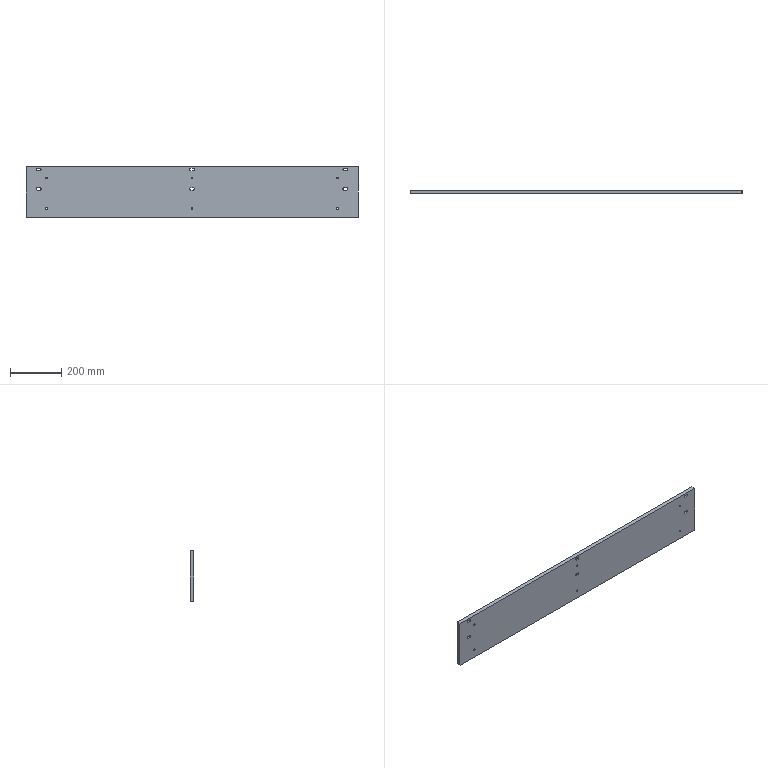Part | NX | features BREP 1 | 1 solid | 76 faces | box 1300 x 15 x 200 mm | volume 3874881 mm3 | plane 40 | cylinder 36 | commonest cylinder face diameters 6.8 x12 10 x12 15 x12